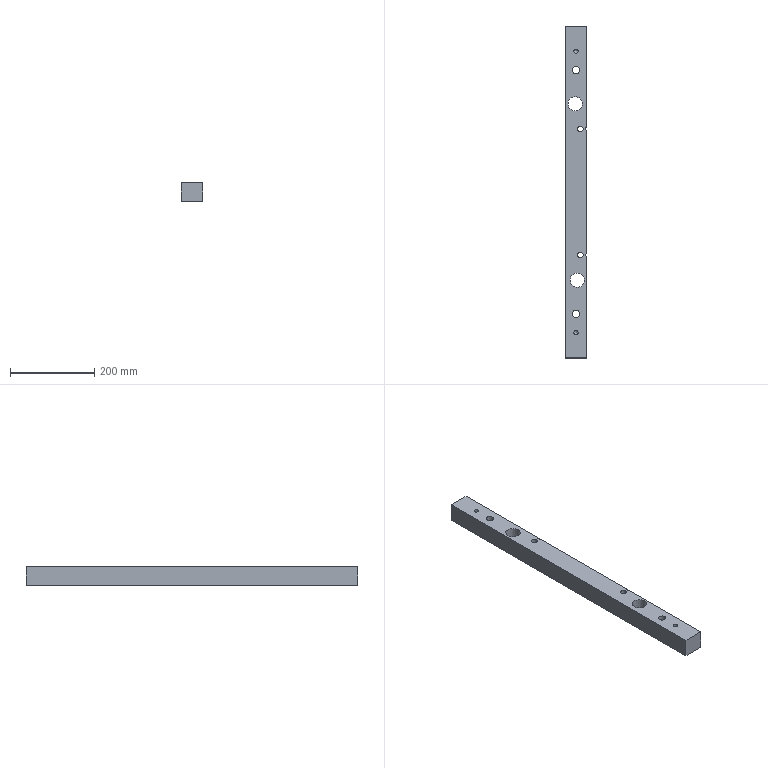Part | STEP file | 015_id2214_x_t | 1 solid | 24 faces | box 50 x 790 x 45 mm | volume 1647676 mm3 | cylinder 12 | plane 8 | cone 4 | commonest cylinder face diameters 14 x6 10.3 x2 17 x2 34 x2